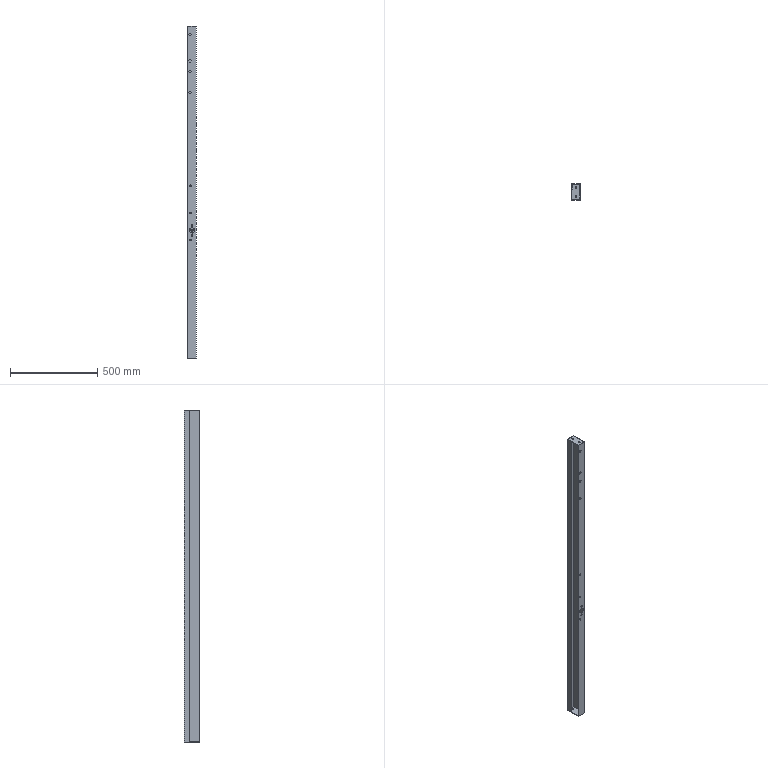Part | SolidWorks | features BaseBody 1 | 1 solid | 61 faces | box 50 x 90 x 1900 mm | volume 1023705 mm3 | plane 39 | cylinder 22 | commonest cylinder face diameters 10.6 x10 11 x8 6.5 x2 30 x2